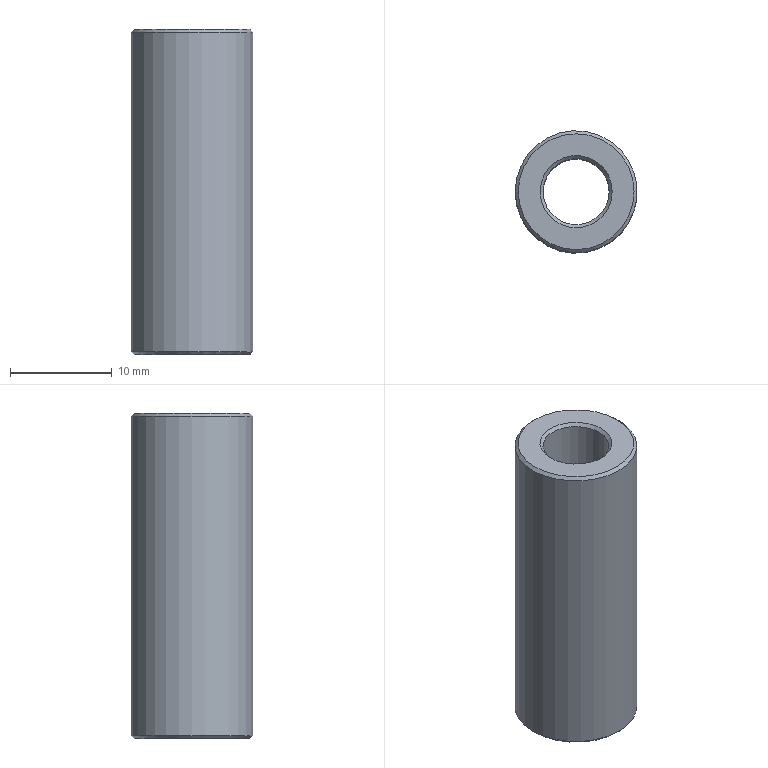Part | STEP file | 1 solid | 8 faces | box 12 x 12 x 32 mm | volume 2552 mm3 | cone 4 | plane 2 | cylinder 2 | commonest cylinder face diameters 6.5 x1 12 x1
STEP:
#1=CARTESIAN_POINT('',(0.,0.,0.));
#2=DIRECTION('',(0.,0.,1.));
#3=DIRECTION('',(1.,0.,0.));
#4=AXIS2_PLACEMENT_3D('',#1,#2,#3);
#5=CARTESIAN_POINT('',(1371.697,494.48,11.619));
#6=VERTEX_POINT('',#5);
#7=CARTESIAN_POINT('',(1375.247,494.48,11.619));
#8=DIRECTION('',(0.,0.,1.));
#9=DIRECTION('',(-1.,0.,0.));
#10=AXIS2_PLACEMENT_3D('',#7,#8,#9);
#11=CIRCLE('',#10,3.55);
#12=CARTESIAN_POINT('',(1375.247,494.48,11.619));
#13=DIRECTION('',(0.,0.,-1.));
#14=DIRECTION('',(-1.,0.,0.));
#15=AXIS2_PLACEMENT_3D('',#12,#13,#14);
#16=PLANE('',#15);
#17=CARTESIAN_POINT('',(3.55,0.));
#18=CARTESIAN_POINT('',(3.55,-6.149));
#19=CARTESIAN_POINT('',(-1.775,-3.074));
#20=CARTESIAN_POINT('',(-7.1,0.));
#21=CARTESIAN_POINT('',(-1.775,3.074));
#22=CARTESIAN_POINT('',(3.55,6.149));
#23=CARTESIAN_POINT('',(3.55,0.));
#24=(BOUNDED_CURVE()B_SPLINE_CURVE(2,(#17,#18,#19,#20,#21,#22,#23),.UNSPECIFIED.,.T.,.F.)B_SPLINE_CURVE_WITH_KNOTS((1,2,2,2,2,1),(-2.094,0.,2.094,4.189,6.283,8.378),.UNSPECIFIED.)CURVE()GEOMETRIC_REPRESENTATION_ITEM()RATIONAL_B_SPLINE_CURVE((1.,0.5,1.,0.5,1.,0.5,1.))REPRESENTATION_ITEM(''));
#25=(GEOMETRIC_REPRESENTATION_CONTEXT(2)PARAMETRIC_REPRESENTATION_CONTEXT()REPRESENTATION_CONTEXT('',''));
#26=DEFINITIONAL_REPRESENTATION('',(#24),#25);
#27=PCURVE('',#16,#26);
#28=CARTESIAN_POINT('',(1375.247,494.48,11.619));
#29=DIRECTION('',(0.,0.,-1.));
#30=DIRECTION('',(-1.,0.,0.));
#31=AXIS2_PLACEMENT_3D('',#28,#29,#30);
#32=CONICAL_SURFACE('',#31,3.55,0.7854);
#33=CARTESIAN_POINT('',(6.283,0.));
#34=DIRECTION('',(-1.,0.));
#35=VECTOR('',#34,1.);
#36=LINE('',#33,#35);
#37=(GEOMETRIC_REPRESENTATION_CONTEXT(2)PARAMETRIC_REPRESENTATION_CONTEXT()REPRESENTATION_CONTEXT('',''));
#38=DEFINITIONAL_REPRESENTATION('',(#36),#37);
#39=PCURVE('',#32,#38);
#40=SURFACE_CURVE('',#11,(#27,#39),.PCURVE_S1.);
#41=EDGE_CURVE('',#6,#6,#40,.T.);
#42=ORIENTED_EDGE('',*,*,#41,.T.);
#43=EDGE_LOOP('',(#42));
#44=FACE_BOUND('',#43,.T.);
#45=CARTESIAN_POINT('',(1369.547,494.48,11.619));
#46=VERTEX_POINT('',#45);
#47=CARTESIAN_POINT('',(1375.247,494.48,11.619));
#48=DIRECTION('',(0.,0.,-1.));
#49=DIRECTION('',(-1.,0.,0.));
#50=AXIS2_PLACEMENT_3D('',#47,#48,#49);
#51=CIRCLE('',#50,5.7);
#52=CARTESIAN_POINT('',(0.,0.));
#53=DIRECTION('',(1.,0.));
#54=AXIS2_PLACEMENT_2D('',#52,#53);
#55=CIRCLE('',#54,5.7);
#56=(GEOMETRIC_REPRESENTATION_CONTEXT(2)PARAMETRIC_REPRESENTATION_CONTEXT()REPRESENTATION_CONTEXT('',''));
#57=DEFINITIONAL_REPRESENTATION('',(#55),#56);
#58=PCURVE('',#16,#57);
#59=CARTESIAN_POINT('',(1375.247,494.48,11.919));
#60=DIRECTION('',(0.,0.,1.));
#61=DIRECTION('',(1.,0.,0.));
#62=AXIS2_PLACEMENT_3D('',#59,#60,#61);
#63=CONICAL_SURFACE('',#62,6.,0.7854);
#64=CARTESIAN_POINT('',(9.425,-0.3));
#65=DIRECTION('',(-1.,0.));
#66=VECTOR('',#65,1.);
#67=LINE('',#64,#66);
#68=(GEOMETRIC_REPRESENTATION_CONTEXT(2)PARAMETRIC_REPRESENTATION_CONTEXT()REPRESENTATION_CONTEXT('',''));
#69=DEFINITIONAL_REPRESENTATION('',(#67),#68);
#70=PCURVE('',#63,#69);
#71=SURFACE_CURVE('',#51,(#58,#70),.PCURVE_S1.);
#72=EDGE_CURVE('',#46,#46,#71,.T.);
#73=ORIENTED_EDGE('',*,*,#72,.T.);
#74=EDGE_LOOP('',(#73));
#75=FACE_BOUND('',#74,.T.);
#76=ADVANCED_FACE('',(#44,#75),#16,.T.);
#77=CARTESIAN_POINT('',(1369.247,494.48,43.319));
#78=VERTEX_POINT('',#77);
#79=CARTESIAN_POINT('',(1375.247,494.48,43.319));
#80=DIRECTION('',(0.,0.,-1.));
#81=DIRECTION('',(-1.,0.,0.));
#82=AXIS2_PLACEMENT_3D('',#79,#80,#81);
#83=CIRCLE('',#82,6.);
#84=CARTESIAN_POINT('',(1375.247,494.48,11.319));
#85=DIRECTION('',(0.,0.,1.));
#86=DIRECTION('',(-1.,0.,0.));
#87=AXIS2_PLACEMENT_3D('',#84,#85,#86);
#88=CYLINDRICAL_SURFACE('',#87,6.);
#89=CARTESIAN_POINT('',(6.283,32.));
#90=DIRECTION('',(-1.,0.));
#91=VECTOR('',#90,1.);
#92=LINE('',#89,#91);
#93=(GEOMETRIC_REPRESENTATION_CONTEXT(2)PARAMETRIC_REPRESENTATION_CONTEXT()REPRESENTATION_CONTEXT('',''));
#94=DEFINITIONAL_REPRESENTATION('',(#92),#93);
#95=PCURVE('',#88,#94);
#96=CARTESIAN_POINT('',(1375.247,494.48,43.319));
#97=DIRECTION('',(0.,0.,-1.));
#98=DIRECTION('',(-1.,0.,0.));
#99=AXIS2_PLACEMENT_3D('',#96,#97,#98);
#100=CONICAL_SURFACE('',#99,6.,0.7854);
#101=CARTESIAN_POINT('',(0.,0.));
#102=DIRECTION('',(1.,0.));
#103=VECTOR('',#102,1.);
#104=LINE('',#101,#103);
#105=(GEOMETRIC_REPRESENTATION_CONTEXT(2)PARAMETRIC_REPRESENTATION_CONTEXT()REPRESENTATION_CONTEXT('',''));
#106=DEFINITIONAL_REPRESENTATION('',(#104),#105);
#107=PCURVE('',#100,#106);
#108=SURFACE_CURVE('',#83,(#95,#107),.PCURVE_S1.);
#109=EDGE_CURVE('',#78,#78,#108,.T.);
#110=ORIENTED_EDGE('',*,*,#109,.T.);
#111=CARTESIAN_POINT('',(1369.247,494.48,11.919));
#112=VERTEX_POINT('',#111);
#113=CARTESIAN_POINT('',(1369.247,494.48,11.919));
#114=CARTESIAN_POINT('',(1369.247,494.48,43.319));
#115=B_SPLINE_CURVE_WITH_KNOTS('',1,(#113,#114),.UNSPECIFIED.,.F.,.F.,(2,2),(0.6,32.),.PIECEWISE_BEZIER_KNOTS.);
#116=CARTESIAN_POINT('',(0.,0.));
#117=DIRECTION('',(0.,1.));
#118=VECTOR('',#117,1.);
#119=LINE('',#116,#118);
#120=(GEOMETRIC_REPRESENTATION_CONTEXT(2)PARAMETRIC_REPRESENTATION_CONTEXT()REPRESENTATION_CONTEXT('',''));
#121=DEFINITIONAL_REPRESENTATION('',(#119),#120);
#122=PCURVE('',#88,#121);
#123=CARTESIAN_POINT('',(6.283,0.));
#124=DIRECTION('',(0.,1.));
#125=VECTOR('',#124,1.);
#126=LINE('',#123,#125);
#127=(GEOMETRIC_REPRESENTATION_CONTEXT(2)PARAMETRIC_REPRESENTATION_CONTEXT()REPRESENTATION_CONTEXT('',''));
#128=DEFINITIONAL_REPRESENTATION('',(#126),#127);
#129=PCURVE('',#88,#128);
#130=SEAM_CURVE('',#115,(#122,#129),.PCURVE_S1.);
#131=EDGE_CURVE('',#112,#78,#130,.T.);
#132=ORIENTED_EDGE('',*,*,#131,.F.);
#133=CARTESIAN_POINT('',(1375.247,494.48,11.919));
#134=DIRECTION('',(0.,0.,1.));
#135=DIRECTION('',(-1.,0.,0.));
#136=AXIS2_PLACEMENT_3D('',#133,#134,#135);
#137=CIRCLE('',#136,6.);
#138=CARTESIAN_POINT('',(0.,0.6));
#139=DIRECTION('',(1.,0.));
#140=VECTOR('',#139,1.);
#141=LINE('',#138,#140);
#142=(GEOMETRIC_REPRESENTATION_CONTEXT(2)PARAMETRIC_REPRESENTATION_CONTEXT()REPRESENTATION_CONTEXT('',''));
#143=DEFINITIONAL_REPRESENTATION('',(#141),#142);
#144=PCURVE('',#88,#143);
#145=CARTESIAN_POINT('',(3.142,0.));
#146=DIRECTION('',(1.,0.));
#147=VECTOR('',#146,1.);
#148=LINE('',#145,#147);
#149=(GEOMETRIC_REPRESENTATION_CONTEXT(2)PARAMETRIC_REPRESENTATION_CONTEXT()REPRESENTATION_CONTEXT('',''));
#150=DEFINITIONAL_REPRESENTATION('',(#148),#149);
#151=PCURVE('',#63,#150);
#152=SURFACE_CURVE('',#137,(#144,#151),.PCURVE_S1.);
#153=EDGE_CURVE('',#112,#112,#152,.T.);
#154=ORIENTED_EDGE('',*,*,#153,.T.);
#155=ORIENTED_EDGE('',*,*,#131,.T.);
#156=EDGE_LOOP('',(#110,#132,#154,#155));
#157=FACE_BOUND('',#156,.T.);
#158=ADVANCED_FACE('',(#157),#88,.T.);
#159=CARTESIAN_POINT('',(1371.697,494.48,43.619));
#160=VERTEX_POINT('',#159);
#161=CARTESIAN_POINT('',(1375.247,494.48,43.619));
#162=DIRECTION('',(0.,0.,-1.));
#163=DIRECTION('',(-1.,0.,0.));
#164=AXIS2_PLACEMENT_3D('',#161,#162,#163);
#165=CIRCLE('',#164,3.55);
#166=CARTESIAN_POINT('',(1375.247,494.48,43.619));
#167=DIRECTION('',(0.,0.,-1.));
#168=DIRECTION('',(-1.,0.,0.));
#169=AXIS2_PLACEMENT_3D('',#166,#167,#168);
#170=PLANE('',#169);
#171=CARTESIAN_POINT('',(0.,0.));
#172=DIRECTION('',(1.,0.));
#173=AXIS2_PLACEMENT_2D('',#171,#172);
#174=CIRCLE('',#173,3.55);
#175=(GEOMETRIC_REPRESENTATION_CONTEXT(2)PARAMETRIC_REPRESENTATION_CONTEXT()REPRESENTATION_CONTEXT('',''));
#176=DEFINITIONAL_REPRESENTATION('',(#174),#175);
#177=PCURVE('',#170,#176);
#178=CARTESIAN_POINT('',(1375.247,494.48,43.619));
#179=DIRECTION('',(0.,0.,1.));
#180=DIRECTION('',(1.,0.,0.));
#181=AXIS2_PLACEMENT_3D('',#178,#179,#180);
#182=CONICAL_SURFACE('',#181,3.55,0.7854);
#183=CARTESIAN_POINT('',(9.425,0.));
#184=DIRECTION('',(-1.,0.));
#185=VECTOR('',#184,1.);
#186=LINE('',#183,#185);
#187=(GEOMETRIC_REPRESENTATION_CONTEXT(2)PARAMETRIC_REPRESENTATION_CONTEXT()REPRESENTATION_CONTEXT('',''));
#188=DEFINITIONAL_REPRESENTATION('',(#186),#187);
#189=PCURVE('',#182,#188);
#190=SURFACE_CURVE('',#165,(#177,#189),.PCURVE_S1.);
#191=EDGE_CURVE('',#160,#160,#190,.T.);
#192=ORIENTED_EDGE('',*,*,#191,.T.);
#193=EDGE_LOOP('',(#192));
#194=FACE_BOUND('',#193,.T.);
#195=CARTESIAN_POINT('',(1369.547,494.48,43.619));
#196=VERTEX_POINT('',#195);
#197=CARTESIAN_POINT('',(1375.247,494.48,43.619));
#198=DIRECTION('',(0.,0.,1.));
#199=DIRECTION('',(-1.,0.,0.));
#200=AXIS2_PLACEMENT_3D('',#197,#198,#199);
#201=CIRCLE('',#200,5.7);
#202=CARTESIAN_POINT('',(5.7,0.));
#203=CARTESIAN_POINT('',(5.7,-9.873));
#204=CARTESIAN_POINT('',(-2.85,-4.936));
#205=CARTESIAN_POINT('',(-11.4,0.));
#206=CARTESIAN_POINT('',(-2.85,4.936));
#207=CARTESIAN_POINT('',(5.7,9.873));
#208=CARTESIAN_POINT('',(5.7,0.));
#209=(BOUNDED_CURVE()B_SPLINE_CURVE(2,(#202,#203,#204,#205,#206,#207,#208),.UNSPECIFIED.,.T.,.F.)B_SPLINE_CURVE_WITH_KNOTS((1,2,2,2,2,1),(-2.094,0.,2.094,4.189,6.283,8.378),.UNSPECIFIED.)CURVE()GEOMETRIC_REPRESENTATION_ITEM()RATIONAL_B_SPLINE_CURVE((1.,0.5,1.,0.5,1.,0.5,1.))REPRESENTATION_ITEM(''));
#210=(GEOMETRIC_REPRESENTATION_CONTEXT(2)PARAMETRIC_REPRESENTATION_CONTEXT()REPRESENTATION_CONTEXT('',''));
#211=DEFINITIONAL_REPRESENTATION('',(#209),#210);
#212=PCURVE('',#170,#211);
#213=CARTESIAN_POINT('',(6.283,-0.3));
#214=DIRECTION('',(-1.,0.));
#215=VECTOR('',#214,1.);
#216=LINE('',#213,#215);
#217=(GEOMETRIC_REPRESENTATION_CONTEXT(2)PARAMETRIC_REPRESENTATION_CONTEXT()REPRESENTATION_CONTEXT('',''));
#218=DEFINITIONAL_REPRESENTATION('',(#216),#217);
#219=PCURVE('',#100,#218);
#220=SURFACE_CURVE('',#201,(#212,#219),.PCURVE_S1.);
#221=EDGE_CURVE('',#196,#196,#220,.T.);
#222=ORIENTED_EDGE('',*,*,#221,.T.);
#223=EDGE_LOOP('',(#222));
#224=FACE_BOUND('',#223,.T.);
#225=ADVANCED_FACE('',(#194,#224),#170,.F.);
#226=CARTESIAN_POINT('',(1371.997,494.48,43.319));
#227=VERTEX_POINT('',#226);
#228=CARTESIAN_POINT('',(1375.247,494.48,43.319));
#229=DIRECTION('',(0.,0.,1.));
#230=DIRECTION('',(-1.,0.,0.));
#231=AXIS2_PLACEMENT_3D('',#228,#229,#230);
#232=CIRCLE('',#231,3.25);
#233=CARTESIAN_POINT('',(1375.247,494.48,11.319));
#234=DIRECTION('',(0.,0.,1.));
#235=DIRECTION('',(1.,0.,0.));
#236=AXIS2_PLACEMENT_3D('',#233,#234,#235);
#237=CYLINDRICAL_SURFACE('',#236,3.25);
#238=CARTESIAN_POINT('',(3.142,32.));
#239=DIRECTION('',(1.,0.));
#240=VECTOR('',#239,1.);
#241=LINE('',#238,#240);
#242=(GEOMETRIC_REPRESENTATION_CONTEXT(2)PARAMETRIC_REPRESENTATION_CONTEXT()REPRESENTATION_CONTEXT('',''));
#243=DEFINITIONAL_REPRESENTATION('',(#241),#242);
#244=PCURVE('',#237,#243);
#245=CARTESIAN_POINT('',(3.142,-0.3));
#246=DIRECTION('',(1.,0.));
#247=VECTOR('',#246,1.);
#248=LINE('',#245,#247);
#249=(GEOMETRIC_REPRESENTATION_CONTEXT(2)PARAMETRIC_REPRESENTATION_CONTEXT()REPRESENTATION_CONTEXT('',''));
#250=DEFINITIONAL_REPRESENTATION('',(#248),#249);
#251=PCURVE('',#182,#250);
#252=SURFACE_CURVE('',#232,(#244,#251),.PCURVE_S1.);
#253=EDGE_CURVE('',#227,#227,#252,.T.);
#254=ORIENTED_EDGE('',*,*,#253,.F.);
#255=CARTESIAN_POINT('',(1371.997,494.48,11.919));
#256=VERTEX_POINT('',#255);
#257=CARTESIAN_POINT('',(1371.997,494.48,11.919));
#258=CARTESIAN_POINT('',(1371.997,494.48,43.319));
#259=B_SPLINE_CURVE_WITH_KNOTS('',1,(#257,#258),.UNSPECIFIED.,.F.,.F.,(2,2),(0.6,32.),.PIECEWISE_BEZIER_KNOTS.);
#260=CARTESIAN_POINT('',(3.142,0.));
#261=DIRECTION('',(0.,1.));
#262=VECTOR('',#261,1.);
#263=LINE('',#260,#262);
#264=(GEOMETRIC_REPRESENTATION_CONTEXT(2)PARAMETRIC_REPRESENTATION_CONTEXT()REPRESENTATION_CONTEXT('',''));
#265=DEFINITIONAL_REPRESENTATION('',(#263),#264);
#266=PCURVE('',#237,#265);
#267=CARTESIAN_POINT('',(9.425,0.));
#268=DIRECTION('',(0.,1.));
#269=VECTOR('',#268,1.);
#270=LINE('',#267,#269);
#271=(GEOMETRIC_REPRESENTATION_CONTEXT(2)PARAMETRIC_REPRESENTATION_CONTEXT()REPRESENTATION_CONTEXT('',''));
#272=DEFINITIONAL_REPRESENTATION('',(#270),#271);
#273=PCURVE('',#237,#272);
#274=SEAM_CURVE('',#259,(#266,#273),.PCURVE_S1.);
#275=EDGE_CURVE('',#256,#227,#274,.T.);
#276=ORIENTED_EDGE('',*,*,#275,.F.);
#277=CARTESIAN_POINT('',(1375.247,494.48,11.919));
#278=DIRECTION('',(0.,0.,-1.));
#279=DIRECTION('',(-1.,0.,0.));
#280=AXIS2_PLACEMENT_3D('',#277,#278,#279);
#281=CIRCLE('',#280,3.25);
#282=CARTESIAN_POINT('',(9.425,0.6));
#283=DIRECTION('',(-1.,0.));
#284=VECTOR('',#283,1.);
#285=LINE('',#282,#284);
#286=(GEOMETRIC_REPRESENTATION_CONTEXT(2)PARAMETRIC_REPRESENTATION_CONTEXT()REPRESENTATION_CONTEXT('',''));
#287=DEFINITIONAL_REPRESENTATION('',(#285),#286);
#288=PCURVE('',#237,#287);
#289=CARTESIAN_POINT('',(0.,-0.3));
#290=DIRECTION('',(1.,0.));
#291=VECTOR('',#290,1.);
#292=LINE('',#289,#291);
#293=(GEOMETRIC_REPRESENTATION_CONTEXT(2)PARAMETRIC_REPRESENTATION_CONTEXT()REPRESENTATION_CONTEXT('',''));
#294=DEFINITIONAL_REPRESENTATION('',(#292),#293);
#295=PCURVE('',#32,#294);
#296=SURFACE_CURVE('',#281,(#288,#295),.PCURVE_S1.);
#297=EDGE_CURVE('',#256,#256,#296,.T.);
#298=ORIENTED_EDGE('',*,*,#297,.F.);
#299=ORIENTED_EDGE('',*,*,#275,.T.);
#300=EDGE_LOOP('',(#254,#276,#298,#299));
#301=FACE_BOUND('',#300,.F.);
#302=ADVANCED_FACE('',(#301),#237,.F.);
#303=ORIENTED_EDGE('',*,*,#297,.T.);
#304=CARTESIAN_POINT('',(1371.997,494.48,11.919));
#305=CARTESIAN_POINT('',(1371.697,494.48,11.619));
#306=B_SPLINE_CURVE_WITH_KNOTS('',1,(#304,#305),.UNSPECIFIED.,.F.,.F.,(2,2),(-0.4243,0.),.PIECEWISE_BEZIER_KNOTS.);
#307=CARTESIAN_POINT('',(6.283,0.));
#308=DIRECTION('',(0.,1.));
#309=VECTOR('',#308,1.);
#310=LINE('',#307,#309);
#311=(GEOMETRIC_REPRESENTATION_CONTEXT(2)PARAMETRIC_REPRESENTATION_CONTEXT()REPRESENTATION_CONTEXT('',''));
#312=DEFINITIONAL_REPRESENTATION('',(#310),#311);
#313=PCURVE('',#32,#312);
#314=CARTESIAN_POINT('',(0.,0.));
#315=DIRECTION('',(0.,1.));
#316=VECTOR('',#315,1.);
#317=LINE('',#314,#316);
#318=(GEOMETRIC_REPRESENTATION_CONTEXT(2)PARAMETRIC_REPRESENTATION_CONTEXT()REPRESENTATION_CONTEXT('',''));
#319=DEFINITIONAL_REPRESENTATION('',(#317),#318);
#320=PCURVE('',#32,#319);
#321=SEAM_CURVE('',#306,(#313,#320),.PCURVE_S1.);
#322=EDGE_CURVE('',#256,#6,#321,.T.);
#323=ORIENTED_EDGE('',*,*,#322,.T.);
#324=ORIENTED_EDGE('',*,*,#41,.T.);
#325=ORIENTED_EDGE('',*,*,#322,.F.);
#326=EDGE_LOOP('',(#303,#323,#324,#325));
#327=FACE_BOUND('',#326,.F.);
#328=ADVANCED_FACE('',(#327),#32,.F.);
#329=ORIENTED_EDGE('',*,*,#72,.F.);
#330=CARTESIAN_POINT('',(1369.547,494.48,11.619));
#331=CARTESIAN_POINT('',(1369.247,494.48,11.919));
#332=B_SPLINE_CURVE_WITH_KNOTS('',1,(#330,#331),.UNSPECIFIED.,.F.,.F.,(2,2),(-0.4243,0.),.PIECEWISE_BEZIER_KNOTS.);
#333=CARTESIAN_POINT('',(9.425,0.));
#334=DIRECTION('',(0.,1.));
#335=VECTOR('',#334,1.);
#336=LINE('',#333,#335);
#337=(GEOMETRIC_REPRESENTATION_CONTEXT(2)PARAMETRIC_REPRESENTATION_CONTEXT()REPRESENTATION_CONTEXT('',''));
#338=DEFINITIONAL_REPRESENTATION('',(#336),#337);
#339=PCURVE('',#63,#338);
#340=CARTESIAN_POINT('',(3.142,0.));
#341=DIRECTION('',(0.,1.));
#342=VECTOR('',#341,1.);
#343=LINE('',#340,#342);
#344=(GEOMETRIC_REPRESENTATION_CONTEXT(2)PARAMETRIC_REPRESENTATION_CONTEXT()REPRESENTATION_CONTEXT('',''));
#345=DEFINITIONAL_REPRESENTATION('',(#343),#344);
#346=PCURVE('',#63,#345);
#347=SEAM_CURVE('',#332,(#339,#346),.PCURVE_S1.);
#348=EDGE_CURVE('',#46,#112,#347,.T.);
#349=ORIENTED_EDGE('',*,*,#348,.T.);
#350=ORIENTED_EDGE('',*,*,#153,.F.);
#351=ORIENTED_EDGE('',*,*,#348,.F.);
#352=EDGE_LOOP('',(#329,#349,#350,#351));
#353=FACE_BOUND('',#352,.T.);
#354=ADVANCED_FACE('',(#353),#63,.T.);
#355=ORIENTED_EDGE('',*,*,#253,.T.);
#356=CARTESIAN_POINT('',(1371.997,494.48,43.319));
#357=CARTESIAN_POINT('',(1371.697,494.48,43.619));
#358=B_SPLINE_CURVE_WITH_KNOTS('',1,(#356,#357),.UNSPECIFIED.,.F.,.F.,(2,2),(-0.4243,0.),.PIECEWISE_BEZIER_KNOTS.);
#359=CARTESIAN_POINT('',(9.425,0.));
#360=DIRECTION('',(0.,1.));
#361=VECTOR('',#360,1.);
#362=LINE('',#359,#361);
#363=(GEOMETRIC_REPRESENTATION_CONTEXT(2)PARAMETRIC_REPRESENTATION_CONTEXT()REPRESENTATION_CONTEXT('',''));
#364=DEFINITIONAL_REPRESENTATION('',(#362),#363);
#365=PCURVE('',#182,#364);
#366=CARTESIAN_POINT('',(3.142,0.));
#367=DIRECTION('',(0.,1.));
#368=VECTOR('',#367,1.);
#369=LINE('',#366,#368);
#370=(GEOMETRIC_REPRESENTATION_CONTEXT(2)PARAMETRIC_REPRESENTATION_CONTEXT()REPRESENTATION_CONTEXT('',''));
#371=DEFINITIONAL_REPRESENTATION('',(#369),#370);
#372=PCURVE('',#182,#371);
#373=SEAM_CURVE('',#358,(#365,#372),.PCURVE_S1.);
#374=EDGE_CURVE('',#227,#160,#373,.T.);
#375=ORIENTED_EDGE('',*,*,#374,.T.);
#376=ORIENTED_EDGE('',*,*,#191,.T.);
#377=ORIENTED_EDGE('',*,*,#374,.F.);
#378=EDGE_LOOP('',(#355,#375,#376,#377));
#379=FACE_BOUND('',#378,.F.);
#380=ADVANCED_FACE('',(#379),#182,.F.);
#381=ORIENTED_EDGE('',*,*,#221,.F.);
#382=CARTESIAN_POINT('',(1369.547,494.48,43.619));
#383=CARTESIAN_POINT('',(1369.247,494.48,43.319));
#384=B_SPLINE_CURVE_WITH_KNOTS('',1,(#382,#383),.UNSPECIFIED.,.F.,.F.,(2,2),(-0.4243,0.),.PIECEWISE_BEZIER_KNOTS.);
#385=CARTESIAN_POINT('',(6.283,0.));
#386=DIRECTION('',(0.,1.));
#387=VECTOR('',#386,1.);
#388=LINE('',#385,#387);
#389=(GEOMETRIC_REPRESENTATION_CONTEXT(2)PARAMETRIC_REPRESENTATION_CONTEXT()REPRESENTATION_CONTEXT('',''));
#390=DEFINITIONAL_REPRESENTATION('',(#388),#389);
#391=PCURVE('',#100,#390);
#392=CARTESIAN_POINT('',(0.,0.));
#393=DIRECTION('',(0.,1.));
#394=VECTOR('',#393,1.);
#395=LINE('',#392,#394);
#396=(GEOMETRIC_REPRESENTATION_CONTEXT(2)PARAMETRIC_REPRESENTATION_CONTEXT()REPRESENTATION_CONTEXT('',''));
#397=DEFINITIONAL_REPRESENTATION('',(#395),#396);
#398=PCURVE('',#100,#397);
#399=SEAM_CURVE('',#384,(#391,#398),.PCURVE_S1.);
#400=EDGE_CURVE('',#196,#78,#399,.T.);
#401=ORIENTED_EDGE('',*,*,#400,.T.);
#402=ORIENTED_EDGE('',*,*,#109,.F.);
#403=ORIENTED_EDGE('',*,*,#400,.F.);
#404=EDGE_LOOP('',(#381,#401,#402,#403));
#405=FACE_BOUND('',#404,.T.);
#406=ADVANCED_FACE('',(#405),#100,.T.);
#407=CLOSED_SHELL('',(#76,#158,#225,#302,#328,#354,#380,#406));
#408=MANIFOLD_SOLID_BREP('',#407);
#409=(LENGTH_UNIT()NAMED_UNIT(*)SI_UNIT(.MILLI.,.METRE.));
#410=UNCERTAINTY_MEASURE_WITH_UNIT(LENGTH_MEASURE(0.00001),#409,'','');
#411=(NAMED_UNIT(*)PLANE_ANGLE_UNIT()SI_UNIT($,.RADIAN.));
#412=(NAMED_UNIT(*)SI_UNIT($,.STERADIAN.)SOLID_ANGLE_UNIT());
#413=(GEOMETRIC_REPRESENTATION_CONTEXT(3)GLOBAL_UNCERTAINTY_ASSIGNED_CONTEXT((#410))GLOBAL_UNIT_ASSIGNED_CONTEXT((#409,#411,#412))REPRESENTATION_CONTEXT('',''));
#414=ADVANCED_BREP_SHAPE_REPRESENTATION('',(#4,#408),#413);